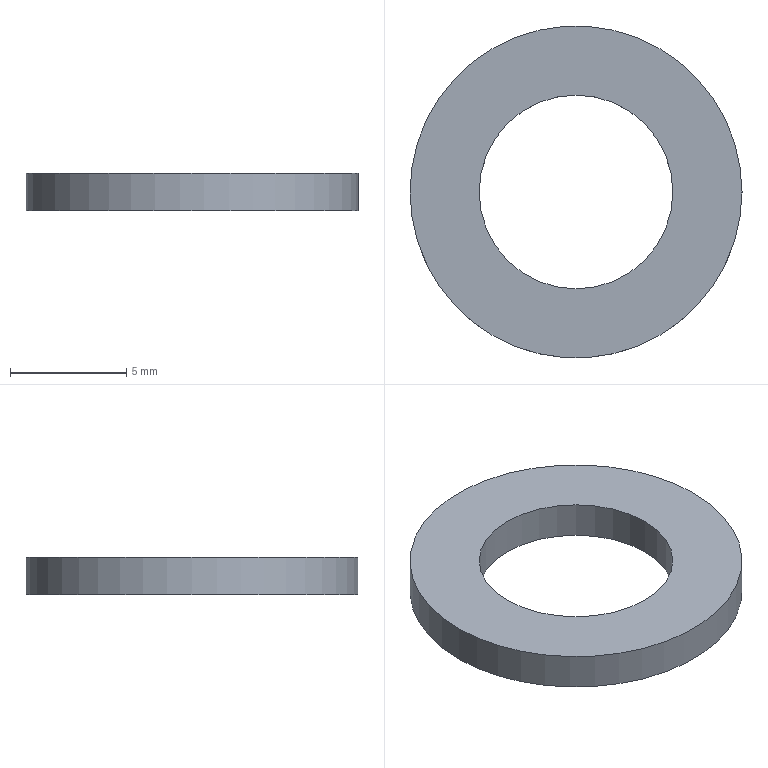Part | NX | features solid 2 | 1 solid | 4 faces | box 14.275 x 14.275 x 1.6 mm | volume 168.864 mm3 | cylinder 2 | plane 2 | commonest cylinder face diameters 8.331 x1 14.275 x1
STEP:
#1=CARTESIAN_POINT('',(7.137,0.,1.6));
#2=VERTEX_POINT('',#1);
#3=CARTESIAN_POINT('',(0.,0.,1.6));
#4=DIRECTION('',(0.,0.,1.));
#5=DIRECTION('',(1.,0.,0.));
#6=AXIS2_PLACEMENT_3D('',#3,#4,#5);
#7=CIRCLE('',#6,7.137);
#8=EDGE_CURVE('',#2,#2,#7,.T.);
#9=ORIENTED_EDGE('',*,*,#8,.F.);
#10=EDGE_LOOP('',(#9));
#11=FACE_BOUND('',#10,.T.);
#12=CARTESIAN_POINT('',(7.137,0.,0.));
#13=VERTEX_POINT('',#12);
#14=CARTESIAN_POINT('',(0.,0.,0.));
#15=DIRECTION('',(0.,0.,1.));
#16=DIRECTION('',(1.,0.,0.));
#17=AXIS2_PLACEMENT_3D('',#14,#15,#16);
#18=CIRCLE('',#17,7.137);
#19=EDGE_CURVE('',#13,#13,#18,.T.);
#20=ORIENTED_EDGE('',*,*,#19,.T.);
#21=EDGE_LOOP('',(#20));
#22=FACE_BOUND('',#21,.T.);
#23=CARTESIAN_POINT('',(0.,0.,1.6));
#24=DIRECTION('',(0.,0.,-1.));
#25=DIRECTION('',(-1.,0.,0.));
#26=AXIS2_PLACEMENT_3D('',#23,#24,#25);
#27=CYLINDRICAL_SURFACE('',#26,7.137);
#28=ADVANCED_FACE('',(#11,#22),#27,.T.);
#29=CARTESIAN_POINT('',(4.166,0.,1.6));
#30=VERTEX_POINT('',#29);
#31=CARTESIAN_POINT('',(0.,0.,1.6));
#32=DIRECTION('',(0.,0.,1.));
#33=DIRECTION('',(1.,0.,0.));
#34=AXIS2_PLACEMENT_3D('',#31,#32,#33);
#35=CIRCLE('',#34,4.166);
#36=EDGE_CURVE('',#30,#30,#35,.T.);
#37=ORIENTED_EDGE('',*,*,#36,.T.);
#38=EDGE_LOOP('',(#37));
#39=FACE_BOUND('',#38,.T.);
#40=CARTESIAN_POINT('',(4.166,0.,0.));
#41=VERTEX_POINT('',#40);
#42=CARTESIAN_POINT('',(0.,0.,0.));
#43=DIRECTION('',(0.,0.,1.));
#44=DIRECTION('',(1.,0.,0.));
#45=AXIS2_PLACEMENT_3D('',#42,#43,#44);
#46=CIRCLE('',#45,4.166);
#47=EDGE_CURVE('',#41,#41,#46,.T.);
#48=ORIENTED_EDGE('',*,*,#47,.F.);
#49=EDGE_LOOP('',(#48));
#50=FACE_BOUND('',#49,.T.);
#51=CARTESIAN_POINT('',(0.,0.,1.6));
#52=DIRECTION('',(0.,0.,-1.));
#53=DIRECTION('',(-1.,0.,0.));
#54=AXIS2_PLACEMENT_3D('',#51,#52,#53);
#55=CYLINDRICAL_SURFACE('',#54,4.166);
#56=ADVANCED_FACE('',(#39,#50),#55,.F.);
#57=ORIENTED_EDGE('',*,*,#8,.T.);
#58=EDGE_LOOP('',(#57));
#59=FACE_BOUND('',#58,.T.);
#60=ORIENTED_EDGE('',*,*,#36,.F.);
#61=EDGE_LOOP('',(#60));
#62=FACE_BOUND('',#61,.T.);
#63=CARTESIAN_POINT('',(0.,0.,1.6));
#64=DIRECTION('',(0.,0.,1.));
#65=DIRECTION('',(1.,0.,0.));
#66=AXIS2_PLACEMENT_3D('',#63,#64,#65);
#67=PLANE('',#66);
#68=ADVANCED_FACE('',(#59,#62),#67,.T.);
#69=ORIENTED_EDGE('',*,*,#19,.F.);
#70=EDGE_LOOP('',(#69));
#71=FACE_BOUND('',#70,.T.);
#72=ORIENTED_EDGE('',*,*,#47,.T.);
#73=EDGE_LOOP('',(#72));
#74=FACE_BOUND('',#73,.T.);
#75=CARTESIAN_POINT('',(0.,0.,0.));
#76=DIRECTION('',(0.,0.,1.));
#77=DIRECTION('',(1.,0.,0.));
#78=AXIS2_PLACEMENT_3D('',#75,#76,#77);
#79=PLANE('',#78);
#80=ADVANCED_FACE('',(#71,#74),#79,.F.);
#81=CLOSED_SHELL('',(#28,#56,#68,#80));
#82=MANIFOLD_SOLID_BREP('',#81);
#83=(LENGTH_UNIT()NAMED_UNIT(*)SI_UNIT(.MILLI.,.METRE.));
#84=UNCERTAINTY_MEASURE_WITH_UNIT(LENGTH_MEASURE(0.00001),#83,'','');
#85=(NAMED_UNIT(*)PLANE_ANGLE_UNIT()SI_UNIT($,.RADIAN.));
#86=(NAMED_UNIT(*)SI_UNIT($,.STERADIAN.)SOLID_ANGLE_UNIT());
#87=(GEOMETRIC_REPRESENTATION_CONTEXT(3)GLOBAL_UNCERTAINTY_ASSIGNED_CONTEXT((#84))GLOBAL_UNIT_ASSIGNED_CONTEXT((#83,#85,#86))REPRESENTATION_CONTEXT('',''));
#88=ADVANCED_BREP_SHAPE_REPRESENTATION('',(#82),#87);